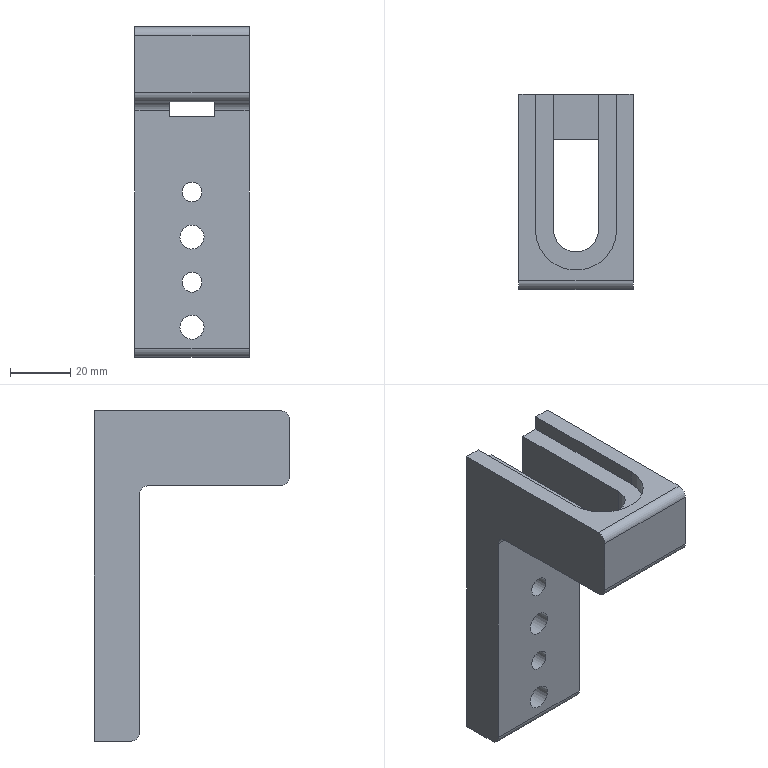Part | STEP file | SN10_008_002_SUPORTE | 1 solid | 25 faces | box 38 x 65 x 110 mm | volume 83544 mm3 | plane 14 | cylinder 11 | commonest cylinder face diameters 6 x5 6.647 x2 8 x2 15 x1 27.1 x1